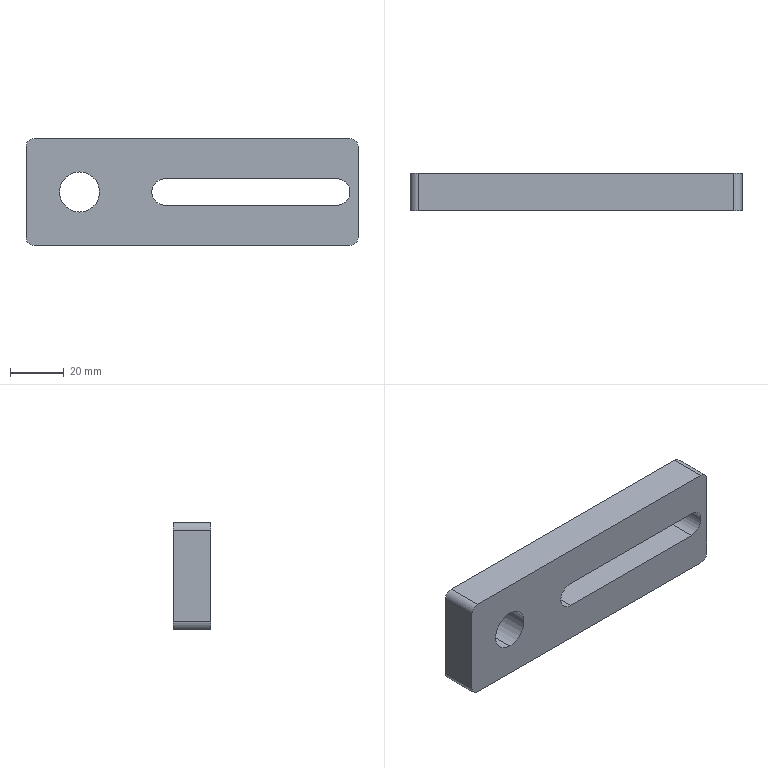Part | SolidWorks | features BaseBody 1 | 1 solid | 16 faces | box 124 x 14 x 40 mm | volume 56798 mm3 | cylinder 8 | plane 8 | commonest cylinder face diameters 6 x4 10 x2 15 x2
STEP:
#1=CARTESIAN_POINT('',(-42.,0.,-7.5));
#2=VERTEX_POINT('',#1);
#3=CARTESIAN_POINT('',(-42.,0.,7.5));
#4=VERTEX_POINT('',#3);
#5=CARTESIAN_POINT('',(-42.,0.,0.));
#6=DIRECTION('',(0.,1.,0.));
#7=DIRECTION('',(0.,0.,1.));
#8=AXIS2_PLACEMENT_3D('',#5,#6,#7);
#9=CIRCLE('',#8,7.5);
#10=EDGE_CURVE('',#2,#4,#9,.T.);
#11=ORIENTED_EDGE('',*,*,#10,.F.);
#12=CARTESIAN_POINT('',(-42.,14.,-7.5));
#13=VERTEX_POINT('',#12);
#14=CARTESIAN_POINT('',(-42.,0.,-7.5));
#15=DIRECTION('',(0.,1.,0.));
#16=VECTOR('',#15,1000.);
#17=LINE('',#14,#16);
#18=EDGE_CURVE('',#2,#13,#17,.T.);
#19=ORIENTED_EDGE('',*,*,#18,.T.);
#20=CARTESIAN_POINT('',(-42.,14.,7.5));
#21=VERTEX_POINT('',#20);
#22=CARTESIAN_POINT('',(-42.,14.,0.));
#23=DIRECTION('',(0.,-1.,0.));
#24=DIRECTION('',(0.,0.,1.));
#25=AXIS2_PLACEMENT_3D('',#22,#23,#24);
#26=CIRCLE('',#25,7.5);
#27=EDGE_CURVE('',#21,#13,#26,.T.);
#28=ORIENTED_EDGE('',*,*,#27,.F.);
#29=CARTESIAN_POINT('',(-42.,0.,7.5));
#30=DIRECTION('',(0.,1.,0.));
#31=VECTOR('',#30,1000.);
#32=LINE('',#29,#31);
#33=EDGE_CURVE('',#4,#21,#32,.T.);
#34=ORIENTED_EDGE('',*,*,#33,.F.);
#35=EDGE_LOOP('',(#11,#19,#28,#34));
#36=FACE_OUTER_BOUND('',#35,.T.);
#37=CARTESIAN_POINT('',(-42.,0.,0.));
#38=DIRECTION('',(0.,1.,0.));
#39=DIRECTION('',(0.,0.,1.));
#40=AXIS2_PLACEMENT_3D('',#37,#38,#39);
#41=CYLINDRICAL_SURFACE('',#40,7.5);
#42=ADVANCED_FACE('',(#36),#41,.F.);
#43=CARTESIAN_POINT('',(-62.,0.,17.));
#44=VERTEX_POINT('',#43);
#45=CARTESIAN_POINT('',(-62.,0.,-17.));
#46=VERTEX_POINT('',#45);
#47=CARTESIAN_POINT('',(-62.,0.,0.));
#48=DIRECTION('',(0.,0.,-1.));
#49=VECTOR('',#48,1000.);
#50=LINE('',#47,#49);
#51=EDGE_CURVE('',#44,#46,#50,.T.);
#52=ORIENTED_EDGE('',*,*,#51,.T.);
#53=CARTESIAN_POINT('',(-59.,0.,-20.));
#54=VERTEX_POINT('',#53);
#55=CARTESIAN_POINT('',(-59.,0.,-17.));
#56=DIRECTION('',(0.,-1.,0.));
#57=DIRECTION('',(0.,0.,-1.));
#58=AXIS2_PLACEMENT_3D('',#55,#56,#57);
#59=CIRCLE('',#58,3.);
#60=EDGE_CURVE('',#46,#54,#59,.T.);
#61=ORIENTED_EDGE('',*,*,#60,.T.);
#62=CARTESIAN_POINT('',(59.,0.,-20.));
#63=VERTEX_POINT('',#62);
#64=CARTESIAN_POINT('',(0.,0.,-20.));
#65=DIRECTION('',(1.,0.,0.));
#66=VECTOR('',#65,1000.);
#67=LINE('',#64,#66);
#68=EDGE_CURVE('',#54,#63,#67,.T.);
#69=ORIENTED_EDGE('',*,*,#68,.T.);
#70=CARTESIAN_POINT('',(62.,0.,-17.));
#71=VERTEX_POINT('',#70);
#72=CARTESIAN_POINT('',(59.,0.,-17.));
#73=DIRECTION('',(0.,-1.,0.));
#74=DIRECTION('',(0.,0.,-1.));
#75=AXIS2_PLACEMENT_3D('',#72,#73,#74);
#76=CIRCLE('',#75,3.);
#77=EDGE_CURVE('',#63,#71,#76,.T.);
#78=ORIENTED_EDGE('',*,*,#77,.T.);
#79=CARTESIAN_POINT('',(62.,0.,17.));
#80=VERTEX_POINT('',#79);
#81=CARTESIAN_POINT('',(62.,0.,0.));
#82=DIRECTION('',(0.,0.,1.));
#83=VECTOR('',#82,1000.);
#84=LINE('',#81,#83);
#85=EDGE_CURVE('',#71,#80,#84,.T.);
#86=ORIENTED_EDGE('',*,*,#85,.T.);
#87=CARTESIAN_POINT('',(59.,0.,20.));
#88=VERTEX_POINT('',#87);
#89=CARTESIAN_POINT('',(59.,0.,17.));
#90=DIRECTION('',(0.,-1.,0.));
#91=DIRECTION('',(0.,0.,-1.));
#92=AXIS2_PLACEMENT_3D('',#89,#90,#91);
#93=CIRCLE('',#92,3.);
#94=EDGE_CURVE('',#80,#88,#93,.T.);
#95=ORIENTED_EDGE('',*,*,#94,.T.);
#96=CARTESIAN_POINT('',(-59.,0.,20.));
#97=VERTEX_POINT('',#96);
#98=CARTESIAN_POINT('',(0.,0.,20.));
#99=DIRECTION('',(-1.,0.,0.));
#100=VECTOR('',#99,1000.);
#101=LINE('',#98,#100);
#102=EDGE_CURVE('',#88,#97,#101,.T.);
#103=ORIENTED_EDGE('',*,*,#102,.T.);
#104=CARTESIAN_POINT('',(-59.,0.,17.));
#105=DIRECTION('',(0.,-1.,0.));
#106=DIRECTION('',(0.,0.,-1.));
#107=AXIS2_PLACEMENT_3D('',#104,#105,#106);
#108=CIRCLE('',#107,3.);
#109=EDGE_CURVE('',#97,#44,#108,.T.);
#110=ORIENTED_EDGE('',*,*,#109,.T.);
#111=EDGE_LOOP('',(#52,#61,#69,#78,#86,#95,#103,#110));
#112=FACE_OUTER_BOUND('',#111,.T.);
#113=CARTESIAN_POINT('',(54.,0.,5.));
#114=VERTEX_POINT('',#113);
#115=CARTESIAN_POINT('',(54.,0.,-5.));
#116=VERTEX_POINT('',#115);
#117=CARTESIAN_POINT('',(54.,0.,0.));
#118=DIRECTION('',(0.,1.,0.));
#119=DIRECTION('',(0.,0.,1.));
#120=AXIS2_PLACEMENT_3D('',#117,#118,#119);
#121=CIRCLE('',#120,5.);
#122=EDGE_CURVE('',#114,#116,#121,.T.);
#123=ORIENTED_EDGE('',*,*,#122,.T.);
#124=CARTESIAN_POINT('',(-10.,0.,-5.));
#125=VERTEX_POINT('',#124);
#126=CARTESIAN_POINT('',(0.,0.,-5.));
#127=DIRECTION('',(-1.,0.,0.));
#128=VECTOR('',#127,1000.);
#129=LINE('',#126,#128);
#130=EDGE_CURVE('',#116,#125,#129,.T.);
#131=ORIENTED_EDGE('',*,*,#130,.T.);
#132=CARTESIAN_POINT('',(-10.,0.,5.));
#133=VERTEX_POINT('',#132);
#134=CARTESIAN_POINT('',(-10.,0.,0.));
#135=DIRECTION('',(0.,1.,0.));
#136=DIRECTION('',(0.,0.,1.));
#137=AXIS2_PLACEMENT_3D('',#134,#135,#136);
#138=CIRCLE('',#137,5.);
#139=EDGE_CURVE('',#125,#133,#138,.T.);
#140=ORIENTED_EDGE('',*,*,#139,.T.);
#141=CARTESIAN_POINT('',(0.,0.,5.));
#142=DIRECTION('',(1.,0.,0.));
#143=VECTOR('',#142,1000.);
#144=LINE('',#141,#143);
#145=EDGE_CURVE('',#133,#114,#144,.T.);
#146=ORIENTED_EDGE('',*,*,#145,.T.);
#147=EDGE_LOOP('',(#123,#131,#140,#146));
#148=FACE_BOUND('',#147,.T.);
#149=CARTESIAN_POINT('',(-42.,0.,0.));
#150=DIRECTION('',(0.,1.,0.));
#151=DIRECTION('',(0.,0.,1.));
#152=AXIS2_PLACEMENT_3D('',#149,#150,#151);
#153=CIRCLE('',#152,7.5);
#154=EDGE_CURVE('',#4,#2,#153,.T.);
#155=ORIENTED_EDGE('',*,*,#154,.T.);
#156=ORIENTED_EDGE('',*,*,#10,.T.);
#157=EDGE_LOOP('',(#155,#156));
#158=FACE_BOUND('',#157,.T.);
#159=CARTESIAN_POINT('',(0.,0.,0.));
#160=DIRECTION('',(0.,-1.,0.));
#161=DIRECTION('',(0.,0.,-1.));
#162=AXIS2_PLACEMENT_3D('',#159,#160,#161);
#163=PLANE('',#162);
#164=ADVANCED_FACE('',(#112,#148,#158),#163,.T.);
#165=ORIENTED_EDGE('',*,*,#60,.F.);
#166=CARTESIAN_POINT('',(-62.,14.,-17.));
#167=VERTEX_POINT('',#166);
#168=CARTESIAN_POINT('',(-62.,14.,-17.));
#169=DIRECTION('',(0.,1.,0.));
#170=VECTOR('',#169,1000.);
#171=LINE('',#168,#170);
#172=EDGE_CURVE('',#46,#167,#171,.T.);
#173=ORIENTED_EDGE('',*,*,#172,.T.);
#174=CARTESIAN_POINT('',(-59.,14.,-20.));
#175=VERTEX_POINT('',#174);
#176=CARTESIAN_POINT('',(-59.,14.,-17.));
#177=DIRECTION('',(0.,-1.,0.));
#178=DIRECTION('',(0.,0.,-1.));
#179=AXIS2_PLACEMENT_3D('',#176,#177,#178);
#180=CIRCLE('',#179,3.);
#181=EDGE_CURVE('',#167,#175,#180,.T.);
#182=ORIENTED_EDGE('',*,*,#181,.T.);
#183=CARTESIAN_POINT('',(-59.,14.,-20.));
#184=DIRECTION('',(0.,-1.,0.));
#185=VECTOR('',#184,1000.);
#186=LINE('',#183,#185);
#187=EDGE_CURVE('',#175,#54,#186,.T.);
#188=ORIENTED_EDGE('',*,*,#187,.T.);
#189=EDGE_LOOP('',(#165,#173,#182,#188));
#190=FACE_OUTER_BOUND('',#189,.T.);
#191=CARTESIAN_POINT('',(-59.,14.,-17.));
#192=DIRECTION('',(0.,-1.,0.));
#193=DIRECTION('',(0.,0.,-1.));
#194=AXIS2_PLACEMENT_3D('',#191,#192,#193);
#195=CYLINDRICAL_SURFACE('',#194,3.);
#196=ADVANCED_FACE('',(#190),#195,.T.);
#197=ORIENTED_EDGE('',*,*,#172,.F.);
#198=ORIENTED_EDGE('',*,*,#51,.F.);
#199=CARTESIAN_POINT('',(-62.,14.,17.));
#200=VERTEX_POINT('',#199);
#201=CARTESIAN_POINT('',(-62.,14.,17.));
#202=DIRECTION('',(0.,-1.,0.));
#203=VECTOR('',#202,1000.);
#204=LINE('',#201,#203);
#205=EDGE_CURVE('',#200,#44,#204,.T.);
#206=ORIENTED_EDGE('',*,*,#205,.F.);
#207=CARTESIAN_POINT('',(-62.,14.,20.));
#208=DIRECTION('',(0.,0.,1.));
#209=VECTOR('',#208,1000.);
#210=LINE('',#207,#209);
#211=EDGE_CURVE('',#167,#200,#210,.T.);
#212=ORIENTED_EDGE('',*,*,#211,.F.);
#213=EDGE_LOOP('',(#197,#198,#206,#212));
#214=FACE_OUTER_BOUND('',#213,.T.);
#215=CARTESIAN_POINT('',(-62.,14.,20.));
#216=DIRECTION('',(1.,0.,0.));
#217=DIRECTION('',(0.,0.,-1.));
#218=AXIS2_PLACEMENT_3D('',#215,#216,#217);
#219=PLANE('',#218);
#220=ADVANCED_FACE('',(#214),#219,.F.);
#221=ORIENTED_EDGE('',*,*,#109,.F.);
#222=CARTESIAN_POINT('',(-59.,14.,20.));
#223=VERTEX_POINT('',#222);
#224=CARTESIAN_POINT('',(-59.,14.,20.));
#225=DIRECTION('',(0.,1.,0.));
#226=VECTOR('',#225,1000.);
#227=LINE('',#224,#226);
#228=EDGE_CURVE('',#97,#223,#227,.T.);
#229=ORIENTED_EDGE('',*,*,#228,.T.);
#230=CARTESIAN_POINT('',(-59.,14.,17.));
#231=DIRECTION('',(0.,-1.,0.));
#232=DIRECTION('',(0.,0.,-1.));
#233=AXIS2_PLACEMENT_3D('',#230,#231,#232);
#234=CIRCLE('',#233,3.);
#235=EDGE_CURVE('',#223,#200,#234,.T.);
#236=ORIENTED_EDGE('',*,*,#235,.T.);
#237=ORIENTED_EDGE('',*,*,#205,.T.);
#238=EDGE_LOOP('',(#221,#229,#236,#237));
#239=FACE_OUTER_BOUND('',#238,.T.);
#240=CARTESIAN_POINT('',(-59.,14.,17.));
#241=DIRECTION('',(0.,-1.,0.));
#242=DIRECTION('',(0.,0.,-1.));
#243=AXIS2_PLACEMENT_3D('',#240,#241,#242);
#244=CYLINDRICAL_SURFACE('',#243,3.);
#245=ADVANCED_FACE('',(#239),#244,.T.);
#246=CARTESIAN_POINT('',(59.,14.,20.));
#247=VERTEX_POINT('',#246);
#248=CARTESIAN_POINT('',(59.,14.,20.));
#249=DIRECTION('',(0.,-1.,0.));
#250=VECTOR('',#249,1000.);
#251=LINE('',#248,#250);
#252=EDGE_CURVE('',#247,#88,#251,.T.);
#253=ORIENTED_EDGE('',*,*,#252,.F.);
#254=CARTESIAN_POINT('',(-62.,14.,20.));
#255=DIRECTION('',(1.,0.,0.));
#256=VECTOR('',#255,1000.);
#257=LINE('',#254,#256);
#258=EDGE_CURVE('',#223,#247,#257,.T.);
#259=ORIENTED_EDGE('',*,*,#258,.F.);
#260=ORIENTED_EDGE('',*,*,#228,.F.);
#261=ORIENTED_EDGE('',*,*,#102,.F.);
#262=EDGE_LOOP('',(#253,#259,#260,#261));
#263=FACE_OUTER_BOUND('',#262,.T.);
#264=CARTESIAN_POINT('',(-62.,14.,20.));
#265=DIRECTION('',(0.,0.,-1.));
#266=DIRECTION('',(-1.,0.,0.));
#267=AXIS2_PLACEMENT_3D('',#264,#265,#266);
#268=PLANE('',#267);
#269=ADVANCED_FACE('',(#263),#268,.F.);
#270=ORIENTED_EDGE('',*,*,#94,.F.);
#271=CARTESIAN_POINT('',(62.,14.,17.));
#272=VERTEX_POINT('',#271);
#273=CARTESIAN_POINT('',(62.,14.,17.));
#274=DIRECTION('',(0.,1.,0.));
#275=VECTOR('',#274,1000.);
#276=LINE('',#273,#275);
#277=EDGE_CURVE('',#80,#272,#276,.T.);
#278=ORIENTED_EDGE('',*,*,#277,.T.);
#279=CARTESIAN_POINT('',(59.,14.,17.));
#280=DIRECTION('',(0.,-1.,0.));
#281=DIRECTION('',(0.,0.,-1.));
#282=AXIS2_PLACEMENT_3D('',#279,#280,#281);
#283=CIRCLE('',#282,3.);
#284=EDGE_CURVE('',#272,#247,#283,.T.);
#285=ORIENTED_EDGE('',*,*,#284,.T.);
#286=ORIENTED_EDGE('',*,*,#252,.T.);
#287=EDGE_LOOP('',(#270,#278,#285,#286));
#288=FACE_OUTER_BOUND('',#287,.T.);
#289=CARTESIAN_POINT('',(59.,14.,17.));
#290=DIRECTION('',(0.,-1.,0.));
#291=DIRECTION('',(0.,0.,-1.));
#292=AXIS2_PLACEMENT_3D('',#289,#290,#291);
#293=CYLINDRICAL_SURFACE('',#292,3.);
#294=ADVANCED_FACE('',(#288),#293,.T.);
#295=CARTESIAN_POINT('',(62.,14.,-17.));
#296=VERTEX_POINT('',#295);
#297=CARTESIAN_POINT('',(62.,14.,-17.));
#298=DIRECTION('',(0.,-1.,0.));
#299=VECTOR('',#298,1000.);
#300=LINE('',#297,#299);
#301=EDGE_CURVE('',#296,#71,#300,.T.);
#302=ORIENTED_EDGE('',*,*,#301,.F.);
#303=CARTESIAN_POINT('',(62.,14.,20.));
#304=DIRECTION('',(0.,0.,-1.));
#305=VECTOR('',#304,1000.);
#306=LINE('',#303,#305);
#307=EDGE_CURVE('',#272,#296,#306,.T.);
#308=ORIENTED_EDGE('',*,*,#307,.F.);
#309=ORIENTED_EDGE('',*,*,#277,.F.);
#310=ORIENTED_EDGE('',*,*,#85,.F.);
#311=EDGE_LOOP('',(#302,#308,#309,#310));
#312=FACE_OUTER_BOUND('',#311,.T.);
#313=CARTESIAN_POINT('',(62.,14.,20.));
#314=DIRECTION('',(-1.,0.,0.));
#315=DIRECTION('',(0.,0.,1.));
#316=AXIS2_PLACEMENT_3D('',#313,#314,#315);
#317=PLANE('',#316);
#318=ADVANCED_FACE('',(#312),#317,.F.);
#319=ORIENTED_EDGE('',*,*,#77,.F.);
#320=CARTESIAN_POINT('',(59.,14.,-20.));
#321=VERTEX_POINT('',#320);
#322=CARTESIAN_POINT('',(59.,14.,-20.));
#323=DIRECTION('',(0.,1.,0.));
#324=VECTOR('',#323,1000.);
#325=LINE('',#322,#324);
#326=EDGE_CURVE('',#63,#321,#325,.T.);
#327=ORIENTED_EDGE('',*,*,#326,.T.);
#328=CARTESIAN_POINT('',(59.,14.,-17.));
#329=DIRECTION('',(0.,-1.,0.));
#330=DIRECTION('',(0.,0.,-1.));
#331=AXIS2_PLACEMENT_3D('',#328,#329,#330);
#332=CIRCLE('',#331,3.);
#333=EDGE_CURVE('',#321,#296,#332,.T.);
#334=ORIENTED_EDGE('',*,*,#333,.T.);
#335=ORIENTED_EDGE('',*,*,#301,.T.);
#336=EDGE_LOOP('',(#319,#327,#334,#335));
#337=FACE_OUTER_BOUND('',#336,.T.);
#338=CARTESIAN_POINT('',(59.,14.,-17.));
#339=DIRECTION('',(0.,-1.,0.));
#340=DIRECTION('',(0.,0.,-1.));
#341=AXIS2_PLACEMENT_3D('',#338,#339,#340);
#342=CYLINDRICAL_SURFACE('',#341,3.);
#343=ADVANCED_FACE('',(#337),#342,.T.);
#344=ORIENTED_EDGE('',*,*,#326,.F.);
#345=ORIENTED_EDGE('',*,*,#68,.F.);
#346=ORIENTED_EDGE('',*,*,#187,.F.);
#347=CARTESIAN_POINT('',(-62.,14.,-20.));
#348=DIRECTION('',(-1.,0.,0.));
#349=VECTOR('',#348,1000.);
#350=LINE('',#347,#349);
#351=EDGE_CURVE('',#321,#175,#350,.T.);
#352=ORIENTED_EDGE('',*,*,#351,.F.);
#353=EDGE_LOOP('',(#344,#345,#346,#352));
#354=FACE_OUTER_BOUND('',#353,.T.);
#355=CARTESIAN_POINT('',(-62.,14.,-20.));
#356=DIRECTION('',(0.,0.,1.));
#357=DIRECTION('',(1.,0.,0.));
#358=AXIS2_PLACEMENT_3D('',#355,#356,#357);
#359=PLANE('',#358);
#360=ADVANCED_FACE('',(#354),#359,.F.);
#361=CARTESIAN_POINT('',(-10.,14.,-5.));
#362=VERTEX_POINT('',#361);
#363=CARTESIAN_POINT('',(-10.,0.,-5.));
#364=DIRECTION('',(0.,1.,0.));
#365=VECTOR('',#364,1000.);
#366=LINE('',#363,#365);
#367=EDGE_CURVE('',#125,#362,#366,.T.);
#368=ORIENTED_EDGE('',*,*,#367,.F.);
#369=ORIENTED_EDGE('',*,*,#130,.F.);
#370=CARTESIAN_POINT('',(54.,14.,-5.));
#371=VERTEX_POINT('',#370);
#372=CARTESIAN_POINT('',(54.,0.,-5.));
#373=DIRECTION('',(0.,-1.,0.));
#374=VECTOR('',#373,1000.);
#375=LINE('',#372,#374);
#376=EDGE_CURVE('',#371,#116,#375,.T.);
#377=ORIENTED_EDGE('',*,*,#376,.F.);
#378=CARTESIAN_POINT('',(-10.,14.,-5.));
#379=DIRECTION('',(1.,0.,0.));
#380=VECTOR('',#379,1000.);
#381=LINE('',#378,#380);
#382=EDGE_CURVE('',#362,#371,#381,.T.);
#383=ORIENTED_EDGE('',*,*,#382,.F.);
#384=EDGE_LOOP('',(#368,#369,#377,#383));
#385=FACE_OUTER_BOUND('',#384,.T.);
#386=CARTESIAN_POINT('',(-10.,0.,-5.));
#387=DIRECTION('',(0.,0.,-1.));
#388=DIRECTION('',(-1.,0.,0.));
#389=AXIS2_PLACEMENT_3D('',#386,#387,#388);
#390=PLANE('',#389);
#391=ADVANCED_FACE('',(#385),#390,.F.);
#392=ORIENTED_EDGE('',*,*,#376,.T.);
#393=ORIENTED_EDGE('',*,*,#122,.F.);
#394=CARTESIAN_POINT('',(54.,14.,5.));
#395=VERTEX_POINT('',#394);
#396=CARTESIAN_POINT('',(54.,0.,5.));
#397=DIRECTION('',(0.,-1.,0.));
#398=VECTOR('',#397,1000.);
#399=LINE('',#396,#398);
#400=EDGE_CURVE('',#395,#114,#399,.T.);
#401=ORIENTED_EDGE('',*,*,#400,.F.);
#402=CARTESIAN_POINT('',(54.,14.,0.));
#403=DIRECTION('',(0.,-1.,0.));
#404=DIRECTION('',(0.,0.,1.));
#405=AXIS2_PLACEMENT_3D('',#402,#403,#404);
#406=CIRCLE('',#405,5.);
#407=EDGE_CURVE('',#371,#395,#406,.T.);
#408=ORIENTED_EDGE('',*,*,#407,.F.);
#409=EDGE_LOOP('',(#392,#393,#401,#408));
#410=FACE_OUTER_BOUND('',#409,.T.);
#411=CARTESIAN_POINT('',(54.,0.,0.));
#412=DIRECTION('',(0.,1.,0.));
#413=DIRECTION('',(0.,0.,1.));
#414=AXIS2_PLACEMENT_3D('',#411,#412,#413);
#415=CYLINDRICAL_SURFACE('',#414,5.);
#416=ADVANCED_FACE('',(#410),#415,.F.);
#417=ORIENTED_EDGE('',*,*,#400,.T.);
#418=ORIENTED_EDGE('',*,*,#145,.F.);
#419=CARTESIAN_POINT('',(-10.,14.,5.));
#420=VERTEX_POINT('',#419);
#421=CARTESIAN_POINT('',(-10.,0.,5.));
#422=DIRECTION('',(0.,-1.,0.));
#423=VECTOR('',#422,1000.);
#424=LINE('',#421,#423);
#425=EDGE_CURVE('',#420,#133,#424,.T.);
#426=ORIENTED_EDGE('',*,*,#425,.F.);
#427=CARTESIAN_POINT('',(-10.,14.,5.));
#428=DIRECTION('',(-1.,0.,0.));
#429=VECTOR('',#428,1000.);
#430=LINE('',#427,#429);
#431=EDGE_CURVE('',#395,#420,#430,.T.);
#432=ORIENTED_EDGE('',*,*,#431,.F.);
#433=EDGE_LOOP('',(#417,#418,#426,#432));
#434=FACE_OUTER_BOUND('',#433,.T.);
#435=CARTESIAN_POINT('',(-10.,0.,5.));
#436=DIRECTION('',(0.,0.,1.));
#437=DIRECTION('',(1.,0.,0.));
#438=AXIS2_PLACEMENT_3D('',#435,#436,#437);
#439=PLANE('',#438);
#440=ADVANCED_FACE('',(#434),#439,.F.);
#441=ORIENTED_EDGE('',*,*,#425,.T.);
#442=ORIENTED_EDGE('',*,*,#139,.F.);
#443=ORIENTED_EDGE('',*,*,#367,.T.);
#444=CARTESIAN_POINT('',(-10.,14.,0.));
#445=DIRECTION('',(0.,-1.,0.));
#446=DIRECTION('',(0.,0.,1.));
#447=AXIS2_PLACEMENT_3D('',#444,#445,#446);
#448=CIRCLE('',#447,5.);
#449=EDGE_CURVE('',#420,#362,#448,.T.);
#450=ORIENTED_EDGE('',*,*,#449,.F.);
#451=EDGE_LOOP('',(#441,#442,#443,#450));
#452=FACE_OUTER_BOUND('',#451,.T.);
#453=CARTESIAN_POINT('',(-10.,0.,0.));
#454=DIRECTION('',(0.,1.,0.));
#455=DIRECTION('',(0.,0.,1.));
#456=AXIS2_PLACEMENT_3D('',#453,#454,#455);
#457=CYLINDRICAL_SURFACE('',#456,5.);
#458=ADVANCED_FACE('',(#452),#457,.F.);
#459=ORIENTED_EDGE('',*,*,#18,.F.);
#460=ORIENTED_EDGE('',*,*,#154,.F.);
#461=ORIENTED_EDGE('',*,*,#33,.T.);
#462=CARTESIAN_POINT('',(-42.,14.,0.));
#463=DIRECTION('',(0.,-1.,0.));
#464=DIRECTION('',(0.,0.,1.));
#465=AXIS2_PLACEMENT_3D('',#462,#463,#464);
#466=CIRCLE('',#465,7.5);
#467=EDGE_CURVE('',#13,#21,#466,.T.);
#468=ORIENTED_EDGE('',*,*,#467,.F.);
#469=EDGE_LOOP('',(#459,#460,#461,#468));
#470=FACE_OUTER_BOUND('',#469,.T.);
#471=CARTESIAN_POINT('',(-42.,0.,0.));
#472=DIRECTION('',(0.,1.,0.));
#473=DIRECTION('',(0.,0.,1.));
#474=AXIS2_PLACEMENT_3D('',#471,#472,#473);
#475=CYLINDRICAL_SURFACE('',#474,7.5);
#476=ADVANCED_FACE('',(#470),#475,.F.);
#477=ORIENTED_EDGE('',*,*,#333,.F.);
#478=ORIENTED_EDGE('',*,*,#351,.T.);
#479=ORIENTED_EDGE('',*,*,#181,.F.);
#480=ORIENTED_EDGE('',*,*,#211,.T.);
#481=ORIENTED_EDGE('',*,*,#235,.F.);
#482=ORIENTED_EDGE('',*,*,#258,.T.);
#483=ORIENTED_EDGE('',*,*,#284,.F.);
#484=ORIENTED_EDGE('',*,*,#307,.T.);
#485=EDGE_LOOP('',(#477,#478,#479,#480,#481,#482,#483,#484));
#486=FACE_OUTER_BOUND('',#485,.T.);
#487=ORIENTED_EDGE('',*,*,#449,.T.);
#488=ORIENTED_EDGE('',*,*,#382,.T.);
#489=ORIENTED_EDGE('',*,*,#407,.T.);
#490=ORIENTED_EDGE('',*,*,#431,.T.);
#491=EDGE_LOOP('',(#487,#488,#489,#490));
#492=FACE_BOUND('',#491,.T.);
#493=ORIENTED_EDGE('',*,*,#27,.T.);
#494=ORIENTED_EDGE('',*,*,#467,.T.);
#495=EDGE_LOOP('',(#493,#494));
#496=FACE_BOUND('',#495,.T.);
#497=CARTESIAN_POINT('',(0.,14.,0.));
#498=DIRECTION('',(0.,-1.,0.));
#499=DIRECTION('',(0.,0.,-1.));
#500=AXIS2_PLACEMENT_3D('',#497,#498,#499);
#501=PLANE('',#500);
#502=ADVANCED_FACE('',(#486,#492,#496),#501,.F.);
#503=CLOSED_SHELL('',(#42,#164,#196,#220,#245,#269,#294,#318,#343,#360,#391,#416,#440,#458,#476,#502));
#504=MANIFOLD_SOLID_BREP('',#503);
#505=CARTESIAN_POINT('',(0.,0.,0.));
#506=DIRECTION('',(0.,0.,1.));
#507=DIRECTION('',(1.,0.,0.));
#508=AXIS2_PLACEMENT_3D('',#505,#506,#507);
#509=(LENGTH_UNIT()NAMED_UNIT(*)SI_UNIT(.MILLI.,.METRE.));
#510=UNCERTAINTY_MEASURE_WITH_UNIT(LENGTH_MEASURE(0.00001),#509,'','');
#511=(NAMED_UNIT(*)PLANE_ANGLE_UNIT()SI_UNIT($,.RADIAN.));
#512=(NAMED_UNIT(*)SI_UNIT($,.STERADIAN.)SOLID_ANGLE_UNIT());
#513=(GEOMETRIC_REPRESENTATION_CONTEXT(3)GLOBAL_UNCERTAINTY_ASSIGNED_CONTEXT((#510))GLOBAL_UNIT_ASSIGNED_CONTEXT((#509,#511,#512))REPRESENTATION_CONTEXT('',''));
#514=ADVANCED_BREP_SHAPE_REPRESENTATION('',(#504,#508),#513);